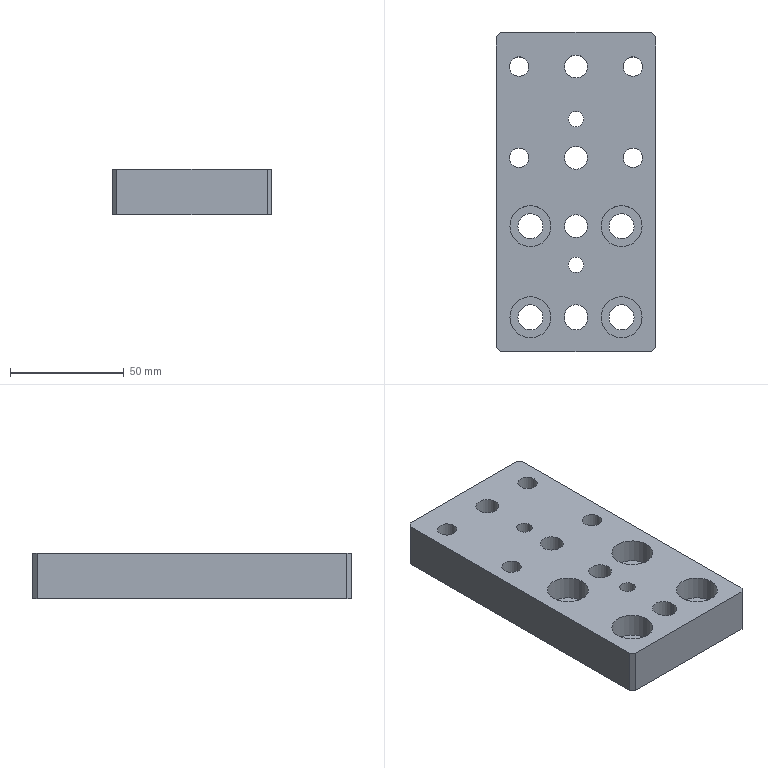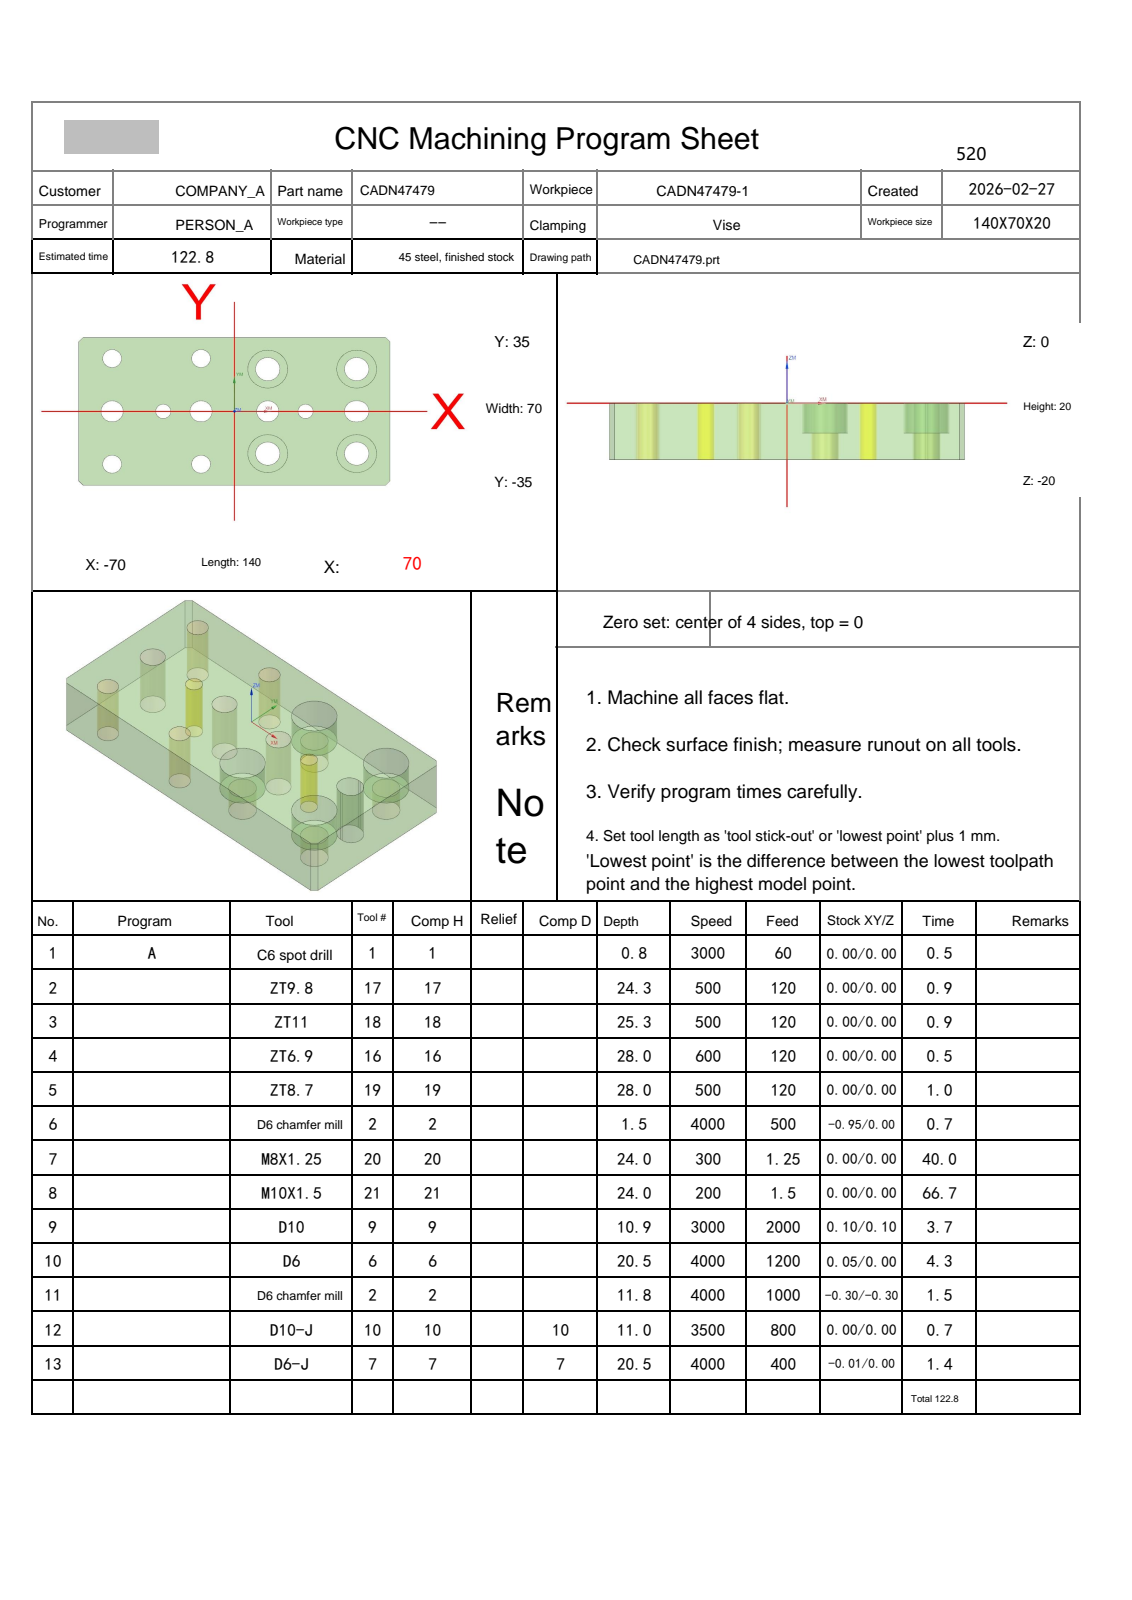NC program | NX | posted by the shop | part box 70 x 140 x 20 mm
Lines 1648 to 3434 of 3634, first 1152 of 1787 lines:
N10 T06 M06
(D6  D=6. R=0. H=06 ce=0.05 di=0.00)
G00 G90 G54 X55. Y1.95 M03 S3500
G43 H06 Z30.
M08
Z.5
G01 X54.5 Z.495 F1200.
G03 X52.55 Y0.0 Z.463 I0.0 J-1.95
X54.5 Y-1.95 Z.43 I1.95 J0.0
G01 X55.5 Z.42
G03 X57.45 Y0.0 Z.388 I0.0 J1.95
X55.5 Y1.95 Z.356 I-1.95 J0.0
G01 X54.5 Z.345
G03 X52.55 Y0.0 Z.313 I0.0 J-1.95
X54.5 Y-1.95 Z.281 I1.95 J0.0
G01 X55.5 Z.27
G03 X57.45 Y0.0 Z.238 I0.0 J1.95
X55.5 Y1.95 Z.206 I-1.95 J0.0
G01 X54.5 Z.195
G03 X52.55 Y0.0 Z.163 I0.0 J-1.95
X54.5 Y-1.95 Z.131 I1.95 J0.0
G01 X55.5 Z.121
G03 X57.45 Y0.0 Z.089 I0.0 J1.95
X55.5 Y1.95 Z.056 I-1.95 J0.0
G01 X54.5 Z.046
G03 X52.55 Y0.0 Z.014 I0.0 J-1.95
X54.5 Y-1.95 Z-.018 I1.95 J0.0
G01 X55.5 Z-.029
G03 X57.45 Y0.0 Z-.061 I0.0 J1.95
X55.5 Y1.95 Z-.093 I-1.95 J0.0
G01 X54.5 Z-.104
G03 X52.55 Y0.0 Z-.136 I0.0 J-1.95
X54.5 Y-1.95 Z-.168 I1.95 J0.0
G01 X55.5 Z-.179
G03 X57.45 Y0.0 Z-.211 I0.0 J1.95
X55.5 Y1.95 Z-.243 I-1.95 J0.0
G01 X54.5 Z-.253
G03 X52.55 Y0.0 Z-.286 I0.0 J-1.95
X54.5 Y-1.95 Z-.318 I1.95 J0.0
G01 X55.5 Z-.328
G03 X57.45 Y0.0 Z-.36 I0.0 J1.95
X55.5 Y1.95 Z-.393 I-1.95 J0.0
G01 X54.5 Z-.403
G03 X52.55 Y0.0 Z-.435 I0.0 J-1.95
X54.5 Y-1.95 Z-.467 I1.95 J0.0
G01 X55.5 Z-.478
G03 X57.45 Y0.0 Z-.51 I0.0 J1.95
X55.5 Y1.95 Z-.542 I-1.95 J0.0
G01 X54.5 Z-.553
G03 X52.55 Y0.0 Z-.585 I0.0 J-1.95
X54.5 Y-1.95 Z-.617 I1.95 J0.0
G01 X55.5 Z-.628
G03 X57.45 Y0.0 Z-.66 I0.0 J1.95
X55.5 Y1.95 Z-.692 I-1.95 J0.0
G01 X54.5 Z-.702
G03 X52.55 Y0.0 Z-.734 I0.0 J-1.95
X54.5 Y-1.95 Z-.767 I1.95 J0.0
G01 X55.5 Z-.777
G03 X57.45 Y0.0 Z-.809 I0.0 J1.95
X55.5 Y1.95 Z-.841 I-1.95 J0.0
G01 X54.5 Z-.852
G03 X52.55 Y0.0 Z-.884 I0.0 J-1.95
X54.5 Y-1.95 Z-.916 I1.95 J0.0
G01 X55.5 Z-.927
G03 X57.45 Y0.0 Z-.959 I0.0 J1.95
X55.5 Y1.95 Z-.991 I-1.95 J0.0
G01 X54.5 Z-1.002
G03 X52.55 Y0.0 Z-1.034 I0.0 J-1.95
X54.5 Y-1.95 Z-1.066 I1.95 J0.0
G01 X55.5 Z-1.076
G03 X57.45 Y0.0 Z-1.109 I0.0 J1.95
X55.5 Y1.95 Z-1.141 I-1.95 J0.0
G01 X54.5 Z-1.151
G03 X52.55 Y0.0 Z-1.183 I0.0 J-1.95
X54.5 Y-1.95 Z-1.216 I1.95 J0.0
G01 X55.5 Z-1.226
G03 X57.45 Y0.0 Z-1.258 I0.0 J1.95
X55.5 Y1.95 Z-1.29 I-1.95 J0.0
G01 X54.5 Z-1.301
G03 X52.55 Y0.0 Z-1.333 I0.0 J-1.95
X54.5 Y-1.95 Z-1.365 I1.95 J0.0
G01 X55.5 Z-1.376
G03 X57.45 Y0.0 Z-1.408 I0.0 J1.95
X55.5 Y1.95 Z-1.44 I-1.95 J0.0
G01 X54.5 Z-1.451
G03 X52.55 Y0.0 Z-1.483 I0.0 J-1.95
X54.5 Y-1.95 Z-1.515 I1.95 J0.0
G01 X55.5 Z-1.525
G03 X57.45 Y0.0 Z-1.557 I0.0 J1.95
X55.5 Y1.95 Z-1.59 I-1.95 J0.0
G01 X54.5 Z-1.6
G03 X52.55 Y0.0 Z-1.632 I0.0 J-1.95
X54.5 Y-1.95 Z-1.664 I1.95 J0.0
G01 X55.5 Z-1.675
G03 X57.45 Y0.0 Z-1.707 I0.0 J1.95
X55.5 Y1.95 Z-1.739 I-1.95 J0.0
G01 X54.5 Z-1.75
G03 X52.55 Y0.0 Z-1.782 I0.0 J-1.95
X54.5 Y-1.95 Z-1.814 I1.95 J0.0
G01 X55.5 Z-1.825
G03 X57.45 Y0.0 Z-1.857 I0.0 J1.95
X55.5 Y1.95 Z-1.889 I-1.95 J0.0
G01 X54.5 Z-1.899
G03 X52.55 Y0.0 Z-1.932 I0.0 J-1.95
X54.5 Y-1.95 Z-1.964 I1.95 J0.0
G01 X55.5 Z-1.974
G03 X57.45 Y0.0 Z-2.006 I0.0 J1.95
X55.5 Y1.95 Z-2.039 I-1.95 J0.0
G01 X54.5 Z-2.049
G03 X52.55 Y0.0 Z-2.081 I0.0 J-1.95
X54.5 Y-1.95 Z-2.113 I1.95 J0.0
G01 X55.5 Z-2.124
G03 X57.45 Y0.0 Z-2.156 I0.0 J1.95
X55.5 Y1.95 Z-2.188 I-1.95 J0.0
G01 X54.5 Z-2.199
G03 X52.55 Y0.0 Z-2.231 I0.0 J-1.95
X54.5 Y-1.95 Z-2.263 I1.95 J0.0
G01 X55.5 Z-2.273
G03 X57.45 Y0.0 Z-2.306 I0.0 J1.95
X55.5 Y1.95 Z-2.338 I-1.95 J0.0
G01 X54.5 Z-2.348
G03 X52.55 Y0.0 Z-2.38 I0.0 J-1.95
X54.5 Y-1.95 Z-2.413 I1.95 J0.0
G01 X55.5 Z-2.423
G03 X57.45 Y0.0 Z-2.455 I0.0 J1.95
X55.5 Y1.95 Z-2.487 I-1.95 J0.0
G01 X54.5 Z-2.498
G03 X52.55 Y0.0 Z-2.53 I0.0 J-1.95
X54.5 Y-1.95 Z-2.562 I1.95 J0.0
G01 X55.5 Z-2.573
G03 X57.45 Y0.0 Z-2.605 I0.0 J1.95
X55.5 Y1.95 Z-2.637 I-1.95 J0.0
G01 X54.5 Z-2.648
G03 X52.55 Y0.0 Z-2.68 I0.0 J-1.95
X54.5 Y-1.95 Z-2.712 I1.95 J0.0
G01 X55.5 Z-2.722
G03 X57.45 Y0.0 Z-2.755 I0.0 J1.95
X55.5 Y1.95 Z-2.787 I-1.95 J0.0
G01 X54.5 Z-2.797
G03 X52.55 Y0.0 Z-2.829 I0.0 J-1.95
X54.5 Y-1.95 Z-2.862 I1.95 J0.0
G01 X55.5 Z-2.872
G03 X57.45 Y0.0 Z-2.904 I0.0 J1.95
X55.5 Y1.95 Z-2.936 I-1.95 J0.0
G01 X54.5 Z-2.947
G03 X52.55 Y0.0 Z-2.979 I0.0 J-1.95
X54.5 Y-1.95 Z-3.011 I1.95 J0.0
G01 X55.5 Z-3.022
G03 X57.45 Y0.0 Z-3.054 I0.0 J1.95
X55.5 Y1.95 Z-3.086 I-1.95 J0.0
G01 X54.5 Z-3.096
G03 X52.55 Y0.0 Z-3.129 I0.0 J-1.95
X54.5 Y-1.95 Z-3.161 I1.95 J0.0
G01 X55.5 Z-3.171
G03 X57.45 Y0.0 Z-3.203 I0.0 J1.95
X55.5 Y1.95 Z-3.236 I-1.95 J0.0
G01 X54.5 Z-3.246
G03 X52.55 Y0.0 Z-3.278 I0.0 J-1.95
X54.5 Y-1.95 Z-3.31 I1.95 J0.0
G01 X55.5 Z-3.321
G03 X57.45 Y0.0 Z-3.353 I0.0 J1.95
X55.5 Y1.95 Z-3.385 I-1.95 J0.0
G01 X54.5 Z-3.396
G03 X52.55 Y0.0 Z-3.428 I0.0 J-1.95
X54.5 Y-1.95 Z-3.46 I1.95 J0.0
G01 X55.5 Z-3.471
G03 X57.45 Y0.0 Z-3.503 I0.0 J1.95
X55.5 Y1.95 Z-3.535 I-1.95 J0.0
G01 X54.5 Z-3.545
G03 X52.55 Y0.0 Z-3.578 I0.0 J-1.95
X54.5 Y-1.95 Z-3.61 I1.95 J0.0
G01 X55.5 Z-3.62
G03 X57.45 Y0.0 Z-3.652 I0.0 J1.95
X55.5 Y1.95 Z-3.685 I-1.95 J0.0
G01 X54.5 Z-3.695
G03 X52.55 Y0.0 Z-3.727 I0.0 J-1.95
X54.5 Y-1.95 Z-3.759 I1.95 J0.0
G01 X55.5 Z-3.77
G03 X57.45 Y0.0 Z-3.802 I0.0 J1.95
X55.5 Y1.95 Z-3.834 I-1.95 J0.0
G01 X54.5 Z-3.845
G03 X52.55 Y0.0 Z-3.877 I0.0 J-1.95
X54.5 Y-1.95 Z-3.909 I1.95 J0.0
G01 X55.5 Z-3.919
G03 X57.45 Y0.0 Z-3.952 I0.0 J1.95
X55.5 Y1.95 Z-3.984 I-1.95 J0.0
G01 X54.5 Z-3.994
G03 X52.55 Y0.0 Z-4.026 I0.0 J-1.95
X54.5 Y-1.95 Z-4.059 I1.95 J0.0
G01 X55.5 Z-4.069
G03 X57.45 Y0.0 Z-4.101 I0.0 J1.95
X55.5 Y1.95 Z-4.133 I-1.95 J0.0
G01 X54.5 Z-4.144
G03 X52.55 Y0.0 Z-4.176 I0.0 J-1.95
X54.5 Y-1.95 Z-4.208 I1.95 J0.0
G01 X55.5 Z-4.219
G03 X57.45 Y0.0 Z-4.251 I0.0 J1.95
X55.5 Y1.95 Z-4.283 I-1.95 J0.0
G01 X54.5 Z-4.294
G03 X52.55 Y0.0 Z-4.326 I0.0 J-1.95
X54.5 Y-1.95 Z-4.358 I1.95 J0.0
G01 X55.5 Z-4.368
G03 X57.45 Y0.0 Z-4.401 I0.0 J1.95
X55.5 Y1.95 Z-4.433 I-1.95 J0.0
G01 X54.5 Z-4.443
G03 X52.55 Y0.0 Z-4.475 I0.0 J-1.95
X54.5 Y-1.95 Z-4.508 I1.95 J0.0
G01 X55.5 Z-4.518
G03 X57.45 Y0.0 Z-4.55 I0.0 J1.95
X55.5 Y1.95 Z-4.582 I-1.95 J0.0
G01 X54.5 Z-4.593
G03 X52.55 Y0.0 Z-4.625 I0.0 J-1.95
X54.5 Y-1.95 Z-4.657 I1.95 J0.0
G01 X55.5 Z-4.668
G03 X57.45 Y0.0 Z-4.7 I0.0 J1.95
X55.5 Y1.95 Z-4.732 I-1.95 J0.0
G01 X54.5 Z-4.742
G03 X52.55 Y0.0 Z-4.775 I0.0 J-1.95
X54.5 Y-1.95 Z-4.807 I1.95 J0.0
G01 X55.5 Z-4.817
G03 X57.45 Y0.0 Z-4.849 I0.0 J1.95
X55.5 Y1.95 Z-4.882 I-1.95 J0.0
G01 X54.5 Z-4.892
G03 X52.55 Y0.0 Z-4.924 I0.0 J-1.95
X54.5 Y-1.95 Z-4.956 I1.95 J0.0
G01 X55.5 Z-4.967
G03 X57.45 Y0.0 Z-4.999 I0.0 J1.95
X55.5 Y1.95 Z-5.031 I-1.95 J0.0
G01 X54.5 Z-5.042
G03 X52.55 Y0.0 Z-5.074 I0.0 J-1.95
X54.5 Y-1.95 Z-5.106 I1.95 J0.0
G01 X55.5 Z-5.117
G03 X57.45 Y0.0 Z-5.149 I0.0 J1.95
X55.5 Y1.95 Z-5.181 I-1.95 J0.0
G01 X54.5 Z-5.191
G03 X52.55 Y0.0 Z-5.224 I0.0 J-1.95
X54.5 Y-1.95 Z-5.256 I1.95 J0.0
G01 X55.5 Z-5.266
G03 X57.45 Y0.0 Z-5.298 I0.0 J1.95
X55.5 Y1.95 Z-5.331 I-1.95 J0.0
G01 X54.5 Z-5.341
G03 X52.55 Y0.0 Z-5.373 I0.0 J-1.95
X54.5 Y-1.95 Z-5.405 I1.95 J0.0
G01 X55.5 Z-5.416
G03 X57.45 Y0.0 Z-5.448 I0.0 J1.95
X55.5 Y1.95 Z-5.48 I-1.95 J0.0
G01 X54.5 Z-5.491
G03 X52.55 Y0.0 Z-5.523 I0.0 J-1.95
X54.5 Y-1.95 Z-5.555 I1.95 J0.0
G01 X55.5 Z-5.565
G03 X57.45 Y0.0 Z-5.598 I0.0 J1.95
X55.5 Y1.95 Z-5.63 I-1.95 J0.0
G01 X54.5 Z-5.64
G03 X52.55 Y0.0 Z-5.672 I0.0 J-1.95
X54.5 Y-1.95 Z-5.705 I1.95 J0.0
G01 X55.5 Z-5.715
G03 X57.45 Y0.0 Z-5.747 I0.0 J1.95
X55.5 Y1.95 Z-5.779 I-1.95 J0.0
G01 X54.5 Z-5.79
G03 X52.55 Y0.0 Z-5.822 I0.0 J-1.95
X54.5 Y-1.95 Z-5.854 I1.95 J0.0
G01 X55.5 Z-5.865
G03 X57.45 Y0.0 Z-5.897 I0.0 J1.95
X55.5 Y1.95 Z-5.929 I-1.95 J0.0
G01 X54.5 Z-5.94
G03 X52.55 Y0.0 Z-5.972 I0.0 J-1.95
X54.5 Y-1.95 Z-6.004 I1.95 J0.0
G01 X55.5 Z-6.014
G03 X57.45 Y0.0 Z-6.047 I0.0 J1.95
X55.5 Y1.95 Z-6.079 I-1.95 J0.0
G01 X54.5 Z-6.089
G03 X52.55 Y0.0 Z-6.121 I0.0 J-1.95
X54.5 Y-1.95 Z-6.154 I1.95 J0.0
G01 X55.5 Z-6.164
G03 X57.45 Y0.0 Z-6.196 I0.0 J1.95
X55.5 Y1.95 Z-6.228 I-1.95 J0.0
G01 X54.5 Z-6.239
G03 X52.55 Y0.0 Z-6.271 I0.0 J-1.95
X54.5 Y-1.95 Z-6.303 I1.95 J0.0
G01 X55.5 Z-6.314
G03 X57.45 Y0.0 Z-6.346 I0.0 J1.95
X55.5 Y1.95 Z-6.378 I-1.95 J0.0
G01 X54.5 Z-6.388
G03 X52.55 Y0.0 Z-6.421 I0.0 J-1.95
X54.5 Y-1.95 Z-6.453 I1.95 J0.0
G01 X55.5 Z-6.463
G03 X57.45 Y0.0 Z-6.495 I0.0 J1.95
X55.5 Y1.95 Z-6.528 I-1.95 J0.0
G01 X54.5 Z-6.538
G03 X52.55 Y0.0 Z-6.57 I0.0 J-1.95
X54.5 Y-1.95 Z-6.602 I1.95 J0.0
G01 X55.5 Z-6.613
G03 X57.45 Y0.0 Z-6.645 I0.0 J1.95
X55.5 Y1.95 Z-6.677 I-1.95 J0.0
G01 X54.5 Z-6.688
G03 X52.55 Y0.0 Z-6.72 I0.0 J-1.95
X54.5 Y-1.95 Z-6.752 I1.95 J0.0
G01 X55.5 Z-6.763
G03 X57.45 Y0.0 Z-6.795 I0.0 J1.95
X55.5 Y1.95 Z-6.827 I-1.95 J0.0
G01 X54.5 Z-6.837
G03 X52.55 Y0.0 Z-6.87 I0.0 J-1.95
X54.5 Y-1.95 Z-6.902 I1.95 J0.0
G01 X55.5 Z-6.912
G03 X57.45 Y0.0 Z-6.944 I0.0 J1.95
X55.5 Y1.95 Z-6.977 I-1.95 J0.0
G01 X54.5 Z-6.987
G03 X52.55 Y0.0 Z-7.019 I0.0 J-1.95
X54.5 Y-1.95 Z-7.051 I1.95 J0.0
G01 X55.5 Z-7.062
G03 X57.45 Y0.0 Z-7.094 I0.0 J1.95
X55.5 Y1.95 Z-7.126 I-1.95 J0.0
G01 X54.5 Z-7.137
G03 X52.55 Y0.0 Z-7.169 I0.0 J-1.95
X54.5 Y-1.95 Z-7.201 I1.95 J0.0
G01 X55.5 Z-7.211
G03 X57.45 Y0.0 Z-7.244 I0.0 J1.95
X55.5 Y1.95 Z-7.276 I-1.95 J0.0
G01 X54.5 Z-7.286
G03 X52.55 Y0.0 Z-7.318 I0.0 J-1.95
X54.5 Y-1.95 Z-7.351 I1.95 J0.0
G01 X55.5 Z-7.361
G03 X57.45 Y0.0 Z-7.393 I0.0 J1.95
X55.5 Y1.95 Z-7.425 I-1.95 J0.0
G01 X54.5 Z-7.436
G03 X52.55 Y0.0 Z-7.468 I0.0 J-1.95
X54.5 Y-1.95 Z-7.5 I1.95 J0.0
G01 X55.5 Z-7.511
G03 X57.45 Y0.0 Z-7.543 I0.0 J1.95
X55.5 Y1.95 Z-7.575 I-1.95 J0.0
G01 X54.5 Z-7.586
G03 X52.55 Y0.0 Z-7.618 I0.0 J-1.95
X54.5 Y-1.95 Z-7.65 I1.95 J0.0
G01 X55.5 Z-7.66
G03 X57.45 Y0.0 Z-7.693 I0.0 J1.95
X55.5 Y1.95 Z-7.725 I-1.95 J0.0
G01 X54.5 Z-7.735
G03 X52.55 Y0.0 Z-7.767 I0.0 J-1.95
X54.5 Y-1.95 Z-7.799 I1.95 J0.0
G01 X55.5 Z-7.81
G03 X57.45 Y0.0 Z-7.842 I0.0 J1.95
X55.5 Y1.95 Z-7.874 I-1.95 J0.0
G01 X54.5 Z-7.885
G03 X52.55 Y0.0 Z-7.917 I0.0 J-1.95
X54.5 Y-1.95 Z-7.949 I1.95 J0.0
G01 X55.5 Z-7.96
G03 X57.45 Y0.0 Z-7.992 I0.0 J1.95
X55.5 Y1.95 Z-8.024 I-1.95 J0.0
G01 X54.5 Z-8.034
G03 X52.55 Y0.0 Z-8.067 I0.0 J-1.95
X54.5 Y-1.95 Z-8.099 I1.95 J0.0
G01 X55.5 Z-8.109
G03 X57.45 Y0.0 Z-8.141 I0.0 J1.95
X55.5 Y1.95 Z-8.174 I-1.95 J0.0
G01 X54.5 Z-8.184
G03 X52.55 Y0.0 Z-8.216 I0.0 J-1.95
X54.5 Y-1.95 Z-8.248 I1.95 J0.0
G01 X55.5 Z-8.259
G03 X57.45 Y0.0 Z-8.291 I0.0 J1.95
X55.5 Y1.95 Z-8.323 I-1.95 J0.0
G01 X54.5 Z-8.334
G03 X52.55 Y0.0 Z-8.366 I0.0 J-1.95
X54.5 Y-1.95 Z-8.398 I1.95 J0.0
G01 X55.5 Z-8.409
G03 X57.45 Y0.0 Z-8.441 I0.0 J1.95
X55.5 Y1.95 Z-8.473 I-1.95 J0.0
G01 X54.5 Z-8.483
G03 X52.55 Y0.0 Z-8.516 I0.0 J-1.95
X54.5 Y-1.95 Z-8.548 I1.95 J0.0
G01 X55.5 Z-8.558
G03 X57.45 Y0.0 Z-8.59 I0.0 J1.95
X55.5 Y1.95 Z-8.622 I-1.95 J0.0
G01 X54.5 Z-8.633
G03 X52.55 Y0.0 Z-8.665 I0.0 J-1.95
X54.5 Y-1.95 Z-8.697 I1.95 J0.0
G01 X55.5 Z-8.708
G03 X57.45 Y0.0 Z-8.74 I0.0 J1.95
X55.5 Y1.95 Z-8.772 I-1.95 J0.0
G01 X54.5 Z-8.783
G03 X52.55 Y0.0 Z-8.815 I0.0 J-1.95
X54.5 Y-1.95 Z-8.847 I1.95 J0.0
G01 X55.5 Z-8.857
G03 X57.45 Y0.0 Z-8.89 I0.0 J1.95
X55.5 Y1.95 Z-8.922 I-1.95 J0.0
G01 X54.5 Z-8.932
G03 X52.55 Y0.0 Z-8.964 I0.0 J-1.95
X54.5 Y-1.95 Z-8.997 I1.95 J0.0
G01 X55.5 Z-9.007
G03 X57.45 Y0.0 Z-9.039 I0.0 J1.95
X55.5 Y1.95 Z-9.071 I-1.95 J0.0
G01 X54.5 Z-9.082
G03 X52.55 Y0.0 Z-9.114 I0.0 J-1.95
X54.5 Y-1.95 Z-9.146 I1.95 J0.0
G01 X55.5 Z-9.157
G03 X57.45 Y0.0 Z-9.189 I0.0 J1.95
X55.5 Y1.95 Z-9.221 I-1.95 J0.0
G01 X54.5 Z-9.232
G03 X52.55 Y0.0 Z-9.264 I0.0 J-1.95
X54.5 Y-1.95 Z-9.296 I1.95 J0.0
G01 X55.5 Z-9.306
G03 X57.45 Y0.0 Z-9.339 I0.0 J1.95
X55.5 Y1.95 Z-9.371 I-1.95 J0.0
G01 X54.5 Z-9.381
G03 X52.55 Y0.0 Z-9.413 I0.0 J-1.95
X54.5 Y-1.95 Z-9.445 I1.95 J0.0
G01 X55.5 Z-9.456
G03 X57.45 Y0.0 Z-9.488 I0.0 J1.95
X55.5 Y1.95 Z-9.52 I-1.95 J0.0
G01 X54.5 Z-9.531
G03 X52.55 Y0.0 Z-9.563 I0.0 J-1.95
X54.5 Y-1.95 Z-9.595 I1.95 J0.0
G01 X55.5 Z-9.606
G03 X57.45 Y0.0 Z-9.638 I0.0 J1.95
X55.5 Y1.95 Z-9.67 I-1.95 J0.0
G01 X54.5 Z-9.68
G03 X52.55 Y0.0 Z-9.713 I0.0 J-1.95
X54.5 Y-1.95 Z-9.745 I1.95 J0.0
G01 X55.5 Z-9.755
G03 X57.45 Y0.0 Z-9.787 I0.0 J1.95
X55.5 Y1.95 Z-9.82 I-1.95 J0.0
G01 X54.5 Z-9.83
G03 X52.55 Y0.0 Z-9.862 I0.0 J-1.95
X54.5 Y-1.95 Z-9.894 I1.95 J0.0
G01 X55.5 Z-9.905
G03 X57.45 Y0.0 Z-9.937 I0.0 J1.95
X55.5 Y1.95 Z-9.969 I-1.95 J0.0
G01 X54.5 Z-9.98
G03 X52.55 Y0.0 Z-10.012 I0.0 J-1.95
X54.5 Y-1.95 Z-10.044 I1.95 J0.0
G01 X55.5 Z-10.055
G03 X57.45 Y0.0 Z-10.087 I0.0 J1.95
X55.5 Y1.95 Z-10.119 I-1.95 J0.0
G01 X54.5 Z-10.129
G03 X52.55 Y0.0 Z-10.161 I0.0 J-1.95
X54.5 Y-1.95 Z-10.194 I1.95 J0.0
G01 X55.5 Z-10.204
G03 X57.45 Y0.0 Z-10.236 I0.0 J1.95
X55.5 Y1.95 Z-10.268 I-1.95 J0.0
G01 X54.5 Z-10.279
G03 X52.55 Y0.0 Z-10.311 I0.0 J-1.95
X54.5 Y-1.95 Z-10.343 I1.95 J0.0
G01 X55.5 Z-10.354
G03 X57.45 Y0.0 Z-10.386 I0.0 J1.95
X55.5 Y1.95 Z-10.418 I-1.95 J0.0
G01 X54.5 Z-10.429
G03 X52.55 Y0.0 Z-10.461 I0.0 J-1.95
X54.5 Y-1.95 Z-10.493 I1.95 J0.0
G01 X55.5 Z-10.503
G03 X57.45 Y0.0 Z-10.536 I0.0 J1.95
X55.5 Y1.95 Z-10.568 I-1.95 J0.0
G01 X54.5 Z-10.578
G03 X52.55 Y0.0 Z-10.61 I0.0 J-1.95
X54.5 Y-1.95 Z-10.643 I1.95 J0.0
G01 X55.5 Z-10.653
G03 X57.45 Y0.0 Z-10.685 I0.0 J1.95
X55.5 Y1.95 Z-10.717 I-1.95 J0.0
G01 X54.5 Z-10.728
G03 X52.55 Y0.0 Z-10.76 I0.0 J-1.95
X54.5 Y-1.95 Z-10.792 I1.95 J0.0
G01 X55.5 Z-10.803
G03 X57.45 Y0.0 Z-10.835 I0.0 J1.95
X55.5 Y1.95 Z-10.867 I-1.95 J0.0
G01 X54.5 Z-10.878
G03 X52.55 Y0.0 Z-10.91 I0.0 J-1.95
X54.5 Y-1.95 Z-10.942 I1.95 J0.0
G01 X55.5 Z-10.952
G03 X57.45 Y0.0 Z-10.984 I0.0 J1.95
X55.5 Y1.95 Z-11.017 I-1.95 J0.0
G01 X54.5 Z-11.027
G03 X52.55 Y0.0 Z-11.059 I0.0 J-1.95
X54.5 Y-1.95 Z-11.091 I1.95 J0.0
G01 X55.5 Z-11.102
G03 X57.45 Y0.0 Z-11.134 I0.0 J1.95
X55.5 Y1.95 Z-11.166 I-1.95 J0.0
G01 X54.5 Z-11.177
G03 X52.55 Y0.0 Z-11.209 I0.0 J-1.95
X54.5 Y-1.95 Z-11.241 I1.95 J0.0
G01 X55.5 Z-11.252
G03 X57.45 Y0.0 Z-11.284 I0.0 J1.95
X55.5 Y1.95 Z-11.316 I-1.95 J0.0
G01 X54.5 Z-11.326
G03 X52.55 Y0.0 Z-11.359 I0.0 J-1.95
X54.5 Y-1.95 Z-11.391 I1.95 J0.0
G01 X55.5 Z-11.401
G03 X57.45 Y0.0 Z-11.433 I0.0 J1.95
X55.5 Y1.95 Z-11.466 I-1.95 J0.0
G01 X54.5 Z-11.476
G03 X52.55 Y0.0 Z-11.508 I0.0 J-1.95
X54.5 Y-1.95 Z-11.54 I1.95 J0.0
G01 X55.5 Z-11.551
G03 X57.45 Y0.0 Z-11.583 I0.0 J1.95
X55.5 Y1.95 Z-11.615 I-1.95 J0.0
G01 X54.5 Z-11.626
G03 X52.55 Y0.0 Z-11.658 I0.0 J-1.95
X54.5 Y-1.95 Z-11.69 I1.95 J0.0
G01 X55.5 Z-11.701
G03 X57.45 Y0.0 Z-11.733 I0.0 J1.95
X55.5 Y1.95 Z-11.765 I-1.95 J0.0
G01 X54.5 Z-11.775
G03 X52.55 Y0.0 Z-11.807 I0.0 J-1.95
X54.5 Y-1.95 Z-11.84 I1.95 J0.0
G01 X55.5 Z-11.85
G03 X57.45 Y0.0 Z-11.882 I0.0 J1.95
X55.5 Y1.95 Z-11.914 I-1.95 J0.0
G01 X54.5 Z-11.925
G03 X52.55 Y0.0 Z-11.957 I0.0 J-1.95
X54.5 Y-1.95 Z-11.989 I1.95 J0.0
G01 X55.5 Z-12.
G03 X57.45 Y0.0 Z-12.032 I0.0 J1.95
X55.5 Y1.95 Z-12.064 I-1.95 J0.0
G01 X54.5 Z-12.075
G03 X52.55 Y0.0 Z-12.107 I0.0 J-1.95
X54.5 Y-1.95 Z-12.139 I1.95 J0.0
G01 X55.5 Z-12.149
G03 X57.45 Y0.0 Z-12.182 I0.0 J1.95
X55.5 Y1.95 Z-12.214 I-1.95 J0.0
G01 X54.5 Z-12.224
G03 X52.55 Y0.0 Z-12.256 I0.0 J-1.95
X54.5 Y-1.95 Z-12.289 I1.95 J0.0
G01 X55.5 Z-12.299
G03 X57.45 Y0.0 Z-12.331 I0.0 J1.95
X55.5 Y1.95 Z-12.363 I-1.95 J0.0
G01 X54.5 Z-12.374
G03 X52.55 Y0.0 Z-12.406 I0.0 J-1.95
X54.5 Y-1.95 Z-12.438 I1.95 J0.0
G01 X55.5 Z-12.449
G03 X57.45 Y0.0 Z-12.481 I0.0 J1.95
X55.5 Y1.95 Z-12.513 I-1.95 J0.0
G01 X54.5 Z-12.523
G03 X52.55 Y0.0 Z-12.556 I0.0 J-1.95
X54.5 Y-1.95 Z-12.588 I1.95 J0.0
G01 X55.5 Z-12.598
G03 X57.45 Y0.0 Z-12.63 I0.0 J1.95
X55.5 Y1.95 Z-12.663 I-1.95 J0.0
G01 X54.5 Z-12.673
G03 X52.55 Y0.0 Z-12.705 I0.0 J-1.95
X54.5 Y-1.95 Z-12.737 I1.95 J0.0
G01 X55.5 Z-12.748
G03 X57.45 Y0.0 Z-12.78 I0.0 J1.95
X55.5 Y1.95 Z-12.812 I-1.95 J0.0
G01 X54.5 Z-12.823
G03 X52.55 Y0.0 Z-12.855 I0.0 J-1.95
X54.5 Y-1.95 Z-12.887 I1.95 J0.0
G01 X55.5 Z-12.898
G03 X57.45 Y0.0 Z-12.93 I0.0 J1.95
X55.5 Y1.95 Z-12.962 I-1.95 J0.0
G01 X54.5 Z-12.972
G03 X52.55 Y0.0 Z-13.005 I0.0 J-1.95
X54.5 Y-1.95 Z-13.037 I1.95 J0.0
G01 X55.5 Z-13.047
G03 X57.45 Y0.0 Z-13.079 I0.0 J1.95
X55.5 Y1.95 Z-13.112 I-1.95 J0.0
G01 X54.5 Z-13.122
G03 X52.55 Y0.0 Z-13.154 I0.0 J-1.95
X54.5 Y-1.95 Z-13.186 I1.95 J0.0
G01 X55.5 Z-13.197
G03 X57.45 Y0.0 Z-13.229 I0.0 J1.95
X55.5 Y1.95 Z-13.261 I-1.95 J0.0
G01 X54.5 Z-13.272
G03 X52.55 Y0.0 Z-13.304 I0.0 J-1.95
X54.5 Y-1.95 Z-13.336 I1.95 J0.0
G01 X55.5 Z-13.346
G03 X57.45 Y0.0 Z-13.379 I0.0 J1.95
X55.5 Y1.95 Z-13.411 I-1.95 J0.0
G01 X54.5 Z-13.421
G03 X52.55 Y0.0 Z-13.453 I0.0 J-1.95
X54.5 Y-1.95 Z-13.486 I1.95 J0.0
G01 X55.5 Z-13.496
G03 X57.45 Y0.0 Z-13.528 I0.0 J1.95
X55.5 Y1.95 Z-13.56 I-1.95 J0.0
G01 X54.5 Z-13.571
G03 X52.55 Y0.0 Z-13.603 I0.0 J-1.95
X54.5 Y-1.95 Z-13.635 I1.95 J0.0
G01 X55.5 Z-13.646
G03 X57.45 Y0.0 Z-13.678 I0.0 J1.95
X55.5 Y1.95 Z-13.71 I-1.95 J0.0
G01 X54.5 Z-13.721
G03 X52.55 Y0.0 Z-13.753 I0.0 J-1.95
X54.5 Y-1.95 Z-13.785 I1.95 J0.0
G01 X55.5 Z-13.795
G03 X57.45 Y0.0 Z-13.828 I0.0 J1.95
X55.5 Y1.95 Z-13.86 I-1.95 J0.0
G01 X54.5 Z-13.87
G03 X52.55 Y0.0 Z-13.902 I0.0 J-1.95
X54.5 Y-1.95 Z-13.935 I1.95 J0.0
G01 X55.5 Z-13.945
G03 X57.45 Y0.0 Z-13.977 I0.0 J1.95
X55.5 Y1.95 Z-14.009 I-1.95 J0.0
G01 X54.5 Z-14.02
G03 X52.55 Y0.0 Z-14.052 I0.0 J-1.95
X54.5 Y-1.95 Z-14.084 I1.95 J0.0
G01 X55.5 Z-14.095
G03 X57.45 Y0.0 Z-14.127 I0.0 J1.95
X55.5 Y1.95 Z-14.159 I-1.95 J0.0
G01 X54.5 Z-14.169
G03 X52.55 Y0.0 Z-14.202 I0.0 J-1.95
X54.5 Y-1.95 Z-14.234 I1.95 J0.0
G01 X55.5 Z-14.244
G03 X57.45 Y0.0 Z-14.276 I0.0 J1.95
X55.5 Y1.95 Z-14.309 I-1.95 J0.0
G01 X54.5 Z-14.319
G03 X52.55 Y0.0 Z-14.351 I0.0 J-1.95
X54.5 Y-1.95 Z-14.383 I1.95 J0.0
G01 X55.5 Z-14.394
G03 X57.45 Y0.0 Z-14.426 I0.0 J1.95
X55.5 Y1.95 Z-14.458 I-1.95 J0.0
G01 X54.5 Z-14.469
G03 X52.55 Y0.0 Z-14.501 I0.0 J-1.95
X54.5 Y-1.95 Z-14.533 I1.95 J0.0
G01 X55.5 Z-14.544
G03 X57.45 Y0.0 Z-14.576 I0.0 J1.95
X55.5 Y1.95 Z-14.608 I-1.95 J0.0
G01 X54.5 Z-14.618
G03 X52.55 Y0.0 Z-14.651 I0.0 J-1.95
X54.5 Y-1.95 Z-14.683 I1.95 J0.0
G01 X55.5 Z-14.693
G03 X57.45 Y0.0 Z-14.725 I0.0 J1.95
X55.5 Y1.95 Z-14.758 I-1.95 J0.0
G01 X54.5 Z-14.768
G03 X52.55 Y0.0 Z-14.8 I0.0 J-1.95
X54.5 Y-1.95 Z-14.832 I1.95 J0.0
G01 X55.5 Z-14.843
G03 X57.45 Y0.0 Z-14.875 I0.0 J1.95
X55.5 Y1.95 Z-14.907 I-1.95 J0.0
G01 X54.5 Z-14.918
G03 X52.55 Y0.0 Z-14.95 I0.0 J-1.95
X54.5 Y-1.95 Z-14.982 I1.95 J0.0
G01 X55.5 Z-14.992
G03 X57.45 Y0.0 Z-15.025 I0.0 J1.95
X55.5 Y1.95 Z-15.057 I-1.95 J0.0
G01 X54.5 Z-15.067
G03 X52.55 Y0.0 Z-15.099 I0.0 J-1.95
X54.5 Y-1.95 Z-15.132 I1.95 J0.0
G01 X55.5 Z-15.142
G03 X57.45 Y0.0 Z-15.174 I0.0 J1.95
X55.5 Y1.95 Z-15.206 I-1.95 J0.0
G01 X54.5 Z-15.217
G03 X52.55 Y0.0 Z-15.249 I0.0 J-1.95
X54.5 Y-1.95 Z-15.281 I1.95 J0.0
G01 X55.5 Z-15.292
G03 X57.45 Y0.0 Z-15.324 I0.0 J1.95
X55.5 Y1.95 Z-15.356 I-1.95 J0.0
G01 X54.5 Z-15.367
G03 X52.55 Y0.0 Z-15.399 I0.0 J-1.95
X54.5 Y-1.95 Z-15.431 I1.95 J0.0
G01 X55.5 Z-15.441
G03 X57.45 Y0.0 Z-15.474 I0.0 J1.95
X55.5 Y1.95 Z-15.506 I-1.95 J0.0
G01 X54.5 Z-15.516
G03 X52.55 Y0.0 Z-15.548 I0.0 J-1.95
X54.5 Y-1.95 Z-15.581 I1.95 J0.0
G01 X55.5 Z-15.591
G03 X57.45 Y0.0 Z-15.623 I0.0 J1.95
X55.5 Y1.95 Z-15.655 I-1.95 J0.0
G01 X54.5 Z-15.666
G03 X52.55 Y0.0 Z-15.698 I0.0 J-1.95
X54.5 Y-1.95 Z-15.73 I1.95 J0.0
G01 X55.5 Z-15.741
G03 X57.45 Y0.0 Z-15.773 I0.0 J1.95
X55.5 Y1.95 Z-15.805 I-1.95 J0.0
G01 X54.5 Z-15.815
G03 X52.55 Y0.0 Z-15.848 I0.0 J-1.95
X54.5 Y-1.95 Z-15.88 I1.95 J0.0
G01 X55.5 Z-15.89
G03 X57.45 Y0.0 Z-15.922 I0.0 J1.95
X55.5 Y1.95 Z-15.955 I-1.95 J0.0
G01 X54.5 Z-15.965
G03 X52.55 Y0.0 Z-15.997 I0.0 J-1.95
X54.5 Y-1.95 Z-16.029 I1.95 J0.0
G01 X55.5 Z-16.04
G03 X57.45 Y0.0 Z-16.072 I0.0 J1.95
X55.5 Y1.95 Z-16.104 I-1.95 J0.0
G01 X54.5 Z-16.115
G03 X52.55 Y0.0 Z-16.147 I0.0 J-1.95
X54.5 Y-1.95 Z-16.179 I1.95 J0.0
G01 X55.5 Z-16.19
G03 X57.45 Y0.0 Z-16.222 I0.0 J1.95
X55.5 Y1.95 Z-16.254 I-1.95 J0.0
G01 X54.5 Z-16.264
G03 X52.55 Y0.0 Z-16.297 I0.0 J-1.95
X54.5 Y-1.95 Z-16.329 I1.95 J0.0
G01 X55.5 Z-16.339
G03 X57.45 Y0.0 Z-16.371 I0.0 J1.95
X55.5 Y1.95 Z-16.404 I-1.95 J0.0
G01 X54.5 Z-16.414
G03 X52.55 Y0.0 Z-16.446 I0.0 J-1.95
X54.5 Y-1.95 Z-16.478 I1.95 J0.0
G01 X55.5 Z-16.489
G03 X57.45 Y0.0 Z-16.521 I0.0 J1.95
X55.5 Y1.95 Z-16.553 I-1.95 J0.0
G01 X54.5 Z-16.564
G03 X52.55 Y0.0 Z-16.596 I0.0 J-1.95
X54.5 Y-1.95 Z-16.628 I1.95 J0.0
G01 X55.5 Z-16.638
G03 X57.45 Y0.0 Z-16.671 I0.0 J1.95
X55.5 Y1.95 Z-16.703 I-1.95 J0.0
G01 X54.5 Z-16.713
G03 X52.55 Y0.0 Z-16.745 I0.0 J-1.95
X54.5 Y-1.95 Z-16.778 I1.95 J0.0
G01 X55.5 Z-16.788
G03 X57.45 Y0.0 Z-16.82 I0.0 J1.95
X55.5 Y1.95 Z-16.852 I-1.95 J0.0
G01 X54.5 Z-16.863
G03 X52.55 Y0.0 Z-16.895 I0.0 J-1.95
X54.5 Y-1.95 Z-16.927 I1.95 J0.0
G01 X55.5 Z-16.938
G03 X57.45 Y0.0 Z-16.97 I0.0 J1.95
X55.5 Y1.95 Z-17.002 I-1.95 J0.0
G01 X54.5 Z-17.013
G03 X52.55 Y0.0 Z-17.045 I0.0 J-1.95
X54.5 Y-1.95 Z-17.077 I1.95 J0.0
G01 X55.5 Z-17.087
G03 X57.45 Y0.0 Z-17.12 I0.0 J1.95
X55.5 Y1.95 Z-17.152 I-1.95 J0.0
G01 X54.5 Z-17.162
G03 X52.55 Y0.0 Z-17.194 I0.0 J-1.95
X54.5 Y-1.95 Z-17.227 I1.95 J0.0
G01 X55.5 Z-17.237
G03 X57.45 Y0.0 Z-17.269 I0.0 J1.95
X55.5 Y1.95 Z-17.301 I-1.95 J0.0
G01 X54.5 Z-17.312
G03 X52.55 Y0.0 Z-17.344 I0.0 J-1.95
X54.5 Y-1.95 Z-17.376 I1.95 J0.0
G01 X55.5 Z-17.387
G03 X57.45 Y0.0 Z-17.419 I0.0 J1.95
X55.5 Y1.95 Z-17.451 I-1.95 J0.0
G01 X54.5 Z-17.461
G03 X52.55 Y0.0 Z-17.494 I0.0 J-1.95
X54.5 Y-1.95 Z-17.526 I1.95 J0.0
G01 X55.5 Z-17.536
G03 X57.45 Y0.0 Z-17.568 I0.0 J1.95
X55.5 Y1.95 Z-17.601 I-1.95 J0.0
G01 X54.5 Z-17.611
G03 X52.55 Y0.0 Z-17.643 I0.0 J-1.95
X54.5 Y-1.95 Z-17.675 I1.95 J0.0
G01 X55.5 Z-17.686
G03 X57.45 Y0.0 Z-17.718 I0.0 J1.95
X55.5 Y1.95 Z-17.75 I-1.95 J0.0
G01 X54.5 Z-17.761
G03 X52.55 Y0.0 Z-17.793 I0.0 J-1.95
X54.5 Y-1.95 Z-17.825 I1.95 J0.0
G01 X55.5 Z-17.836
G03 X57.45 Y0.0 Z-17.868 I0.0 J1.95
X55.5 Y1.95 Z-17.9 I-1.95 J0.0
G01 X54.5 Z-17.91
G03 X52.55 Y0.0 Z-17.943 I0.0 J-1.95
X54.5 Y-1.95 Z-17.975 I1.95 J0.0
G01 X55.5 Z-17.985
G03 X57.45 Y0.0 Z-18.017 I0.0 J1.95
X55.5 Y1.95 Z-18.049 I-1.95 J0.0
G01 X54.5 Z-18.06
G03 X52.55 Y0.0 Z-18.092 I0.0 J-1.95
X54.5 Y-1.95 Z-18.124 I1.95 J0.0
G01 X55.5 Z-18.135
G03 X57.45 Y0.0 Z-18.167 I0.0 J1.95
X55.5 Y1.95 Z-18.199 I-1.95 J0.0
G01 X54.5 Z-18.21
G03 X52.55 Y0.0 Z-18.242 I0.0 J-1.95
X54.5 Y-1.95 Z-18.274 I1.95 J0.0
G01 X55.5 Z-18.284
G03 X57.45 Y0.0 Z-18.317 I0.0 J1.95
X55.5 Y1.95 Z-18.349 I-1.95 J0.0
G01 X54.5 Z-18.359
G03 X52.55 Y0.0 Z-18.391 I0.0 J-1.95
X54.5 Y-1.95 Z-18.424 I1.95 J0.0
G01 X55.5 Z-18.434
G03 X57.45 Y0.0 Z-18.466 I0.0 J1.95
X55.5 Y1.95 Z-18.498 I-1.95 J0.0
G01 X54.5 Z-18.509
G03 X52.55 Y0.0 Z-18.541 I0.0 J-1.95
X54.5 Y-1.95 Z-18.573 I1.95 J0.0
G01 X55.5 Z-18.584
G03 X57.45 Y0.0 Z-18.616 I0.0 J1.95
X55.5 Y1.95 Z-18.648 I-1.95 J0.0
G01 X54.5 Z-18.659
G03 X52.55 Y0.0 Z-18.691 I0.0 J-1.95
X54.5 Y-1.95 Z-18.723 I1.95 J0.0
G01 X55.5 Z-18.733
G03 X57.45 Y0.0 Z-18.766 I0.0 J1.95
X55.5 Y1.95 Z-18.798 I-1.95 J0.0
G01 X54.5 Z-18.808
G03 X52.55 Y0.0 Z-18.84 I0.0 J-1.95
X54.5 Y-1.95 Z-18.872 I1.95 J0.0
G01 X55.5 Z-18.883
G03 X57.45 Y0.0 Z-18.915 I0.0 J1.95
X55.5 Y1.95 Z-18.947 I-1.95 J0.0
G01 X54.5 Z-18.958
G03 X52.55 Y0.0 Z-18.99 I0.0 J-1.95
X54.5 Y-1.95 Z-19.022 I1.95 J0.0
G01 X55.5 Z-19.033
G03 X57.45 Y0.0 Z-19.065 I0.0 J1.95
X55.5 Y1.95 Z-19.097 I-1.95 J0.0
G01 X54.5 Z-19.107
G03 X52.55 Y0.0 Z-19.14 I0.0 J-1.95
X54.5 Y-1.95 Z-19.172 I1.95 J0.0
G01 X55.5 Z-19.182
G03 X57.45 Y0.0 Z-19.214 I0.0 J1.95
X55.5 Y1.95 Z-19.247 I-1.95 J0.0
G01 X54.5 Z-19.257
G03 X52.55 Y0.0 Z-19.289 I0.0 J-1.95
X54.5 Y-1.95 Z-19.321 I1.95 J0.0
G01 X55.5 Z-19.332
G03 X57.45 Y0.0 Z-19.364 I0.0 J1.95
X55.5 Y1.95 Z-19.396 I-1.95 J0.0
G01 X54.5 Z-19.407
G03 X52.55 Y0.0 Z-19.439 I0.0 J-1.95
X54.5 Y-1.95 Z-19.471 I1.95 J0.0
G01 X55.5 Z-19.482
G03 X57.45 Y0.0 Z-19.514 I0.0 J1.95
X55.5 Y1.95 Z-19.546 I-1.95 J0.0
G01 X54.5 Z-19.556
G03 X52.55 Y0.0 Z-19.589 I0.0 J-1.95
X54.5 Y-1.95 Z-19.621 I1.95 J0.0
G01 X55.5 Z-19.631
G03 X57.45 Y0.0 Z-19.663 I0.0 J1.95
X55.5 Y1.95 Z-19.695 I-1.95 J0.0
G01 X54.5 Z-19.706
G03 X52.55 Y0.0 Z-19.738 I0.0 J-1.95
X54.5 Y-1.95 Z-19.77 I1.95 J0.0
G01 X55.5 Z-19.781
G03 X57.45 Y0.0 Z-19.813 I0.0 J1.95
X55.5 Y1.95 Z-19.845 I-1.95 J0.0
G01 X54.5 Z-19.856
G03 X52.55 Y0.0 Z-19.888 I0.0 J-1.95
X54.5 Y-1.95 Z-19.92 I1.95 J0.0
G01 X55.5 Z-19.93
G03 X57.45 Y0.0 Z-19.963 I0.0 J1.95
X55.5 Y1.95 Z-19.995 I-1.95 J0.0
G01 X55. Z-20.
X54.5
G03 X52.55 Y0.0 I0.0 J-1.95
X54.5 Y-1.95 I1.95 J0.0
G01 X55.5
G03 X57.45 Y0.0 I0.0 J1.95
X55.5 Y1.95 I-1.95 J0.0
G01 X55.
X54.5
Z-19.
G00 Z30.
G00 G90 X-55. Y0.0 M03 S4000
Z30.
Z.5
G03 X-54.03 Y.97 I0.0 J.97 F1200.
X-55. Y1.94 I-.97 J0.0
X-55. Y1.94 Z.25 I0.0 J-1.94
X-55. Y1.94 Z0.0 I0.0 J-1.94
X-55. Y1.94 Z-.25 I0.0 J-1.94
X-55. Y1.94 Z-.5 I0.0 J-1.94
X-55. Y1.94 Z-.75 I0.0 J-1.94
X-55. Y1.94 Z-1. I0.0 J-1.94
X-55. Y1.94 Z-1.25 I0.0 J-1.94
X-55. Y1.94 Z-1.5 I0.0 J-1.94
X-55. Y1.94 Z-1.75 I0.0 J-1.94
X-55. Y1.94 Z-2. I0.0 J-1.94
X-55. Y1.94 Z-2.25 I0.0 J-1.94
X-55. Y1.94 Z-2.5 I0.0 J-1.94
X-55. Y1.94 Z-2.75 I0.0 J-1.94
X-55. Y1.94 Z-3. I0.0 J-1.94
X-55. Y1.94 Z-3.25 I0.0 J-1.94
X-55. Y1.94 Z-3.5 I0.0 J-1.94
X-55. Y1.94 Z-3.75 I0.0 J-1.94
X-55. Y1.94 Z-4. I0.0 J-1.94
X-55. Y1.94 Z-4.25 I0.0 J-1.94
X-55. Y1.94 Z-4.5 I0.0 J-1.94
X-55. Y1.94 Z-4.75 I0.0 J-1.94
X-55. Y1.94 Z-5. I0.0 J-1.94
X-55. Y1.94 Z-5.25 I0.0 J-1.94
X-55. Y1.94 Z-5.5 I0.0 J-1.94
X-55. Y1.94 Z-5.75 I0.0 J-1.94
X-55. Y1.94 Z-6. I0.0 J-1.94
X-55. Y1.94 Z-6.25 I0.0 J-1.94
X-55. Y1.94 Z-6.5 I0.0 J-1.94
X-55. Y1.94 Z-6.75 I0.0 J-1.94
X-55. Y1.94 Z-7. I0.0 J-1.94
X-55. Y1.94 Z-7.25 I0.0 J-1.94
X-55. Y1.94 Z-7.5 I0.0 J-1.94
X-55. Y1.94 Z-7.75 I0.0 J-1.94
X-55. Y1.94 Z-8. I0.0 J-1.94
X-55. Y1.94 Z-8.25 I0.0 J-1.94
X-55. Y1.94 Z-8.5 I0.0 J-1.94
X-55. Y1.94 Z-8.75 I0.0 J-1.94
X-55. Y1.94 Z-9. I0.0 J-1.94
X-55. Y1.94 Z-9.25 I0.0 J-1.94
X-55. Y1.94 Z-9.5 I0.0 J-1.94
X-55. Y1.94 Z-9.75 I0.0 J-1.94
X-55. Y1.94 Z-10. I0.0 J-1.94
X-55. Y1.94 Z-10.25 I0.0 J-1.94
X-55. Y1.94 Z-10.5 I0.0 J-1.94
X-55. Y1.94 Z-10.75 I0.0 J-1.94
X-55. Y1.94 Z-11. I0.0 J-1.94
X-55. Y1.94 Z-11.25 I0.0 J-1.94
X-55. Y1.94 Z-11.5 I0.0 J-1.94
X-55. Y1.94 Z-11.75 I0.0 J-1.94
X-55. Y1.94 Z-12. I0.0 J-1.94
X-55. Y1.94 Z-12.25 I0.0 J-1.94
X-55. Y1.94 Z-12.5 I0.0 J-1.94
X-55. Y1.94 Z-12.75 I0.0 J-1.94
X-55. Y1.94 Z-13. I0.0 J-1.94
X-55. Y1.94 Z-13.25 I0.0 J-1.94
X-55. Y1.94 Z-13.5 I0.0 J-1.94
X-55. Y1.94 Z-13.75 I0.0 J-1.94
X-55. Y1.94 Z-14. I0.0 J-1.94
X-55. Y1.94 Z-14.25 I0.0 J-1.94
X-55. Y1.94 Z-14.5 I0.0 J-1.94
X-55. Y1.94 Z-14.75 I0.0 J-1.94
X-55. Y1.94 Z-15. I0.0 J-1.94
X-55. Y1.94 Z-15.25 I0.0 J-1.94
X-55. Y1.94 Z-15.5 I0.0 J-1.94
X-55. Y1.94 Z-15.75 I0.0 J-1.94
X-55. Y1.94 Z-16. I0.0 J-1.94
X-55. Y1.94 Z-16.25 I0.0 J-1.94
X-55. Y1.94 Z-16.5 I0.0 J-1.94
X-55. Y1.94 Z-16.75 I0.0 J-1.94
X-55. Y1.94 Z-17. I0.0 J-1.94
X-55. Y1.94 Z-17.25 I0.0 J-1.94
X-55. Y1.94 Z-17.5 I0.0 J-1.94
X-55. Y1.94 Z-17.75 I0.0 J-1.94
X-55. Y1.94 Z-18. I0.0 J-1.94
X-55. Y1.94 Z-18.25 I0.0 J-1.94
X-55. Y1.94 Z-18.5 I0.0 J-1.94
X-55. Y1.94 Z-18.75 I0.0 J-1.94
X-55. Y1.94 Z-19. I0.0 J-1.94
X-55. Y1.94 Z-19.25 I0.0 J-1.94
X-55. Y1.94 Z-19.5 I0.0 J-1.94
X-55. Y1.94 Z-19.75 I0.0 J-1.94
X-55. Y1.94 Z-20. I0.0 J-1.94
X-55. Y1.94 Z-20.25 I0.0 J-1.94
X-55. Y1.94 Z-20.5 I0.0 J-1.94
X-56.94 Y0.0 I0.0 J-1.94
X-55. Y-1.94 I1.94 J0.0
X-53.06 Y0.0 I0.0 J1.94
X-55. Y1.94 I-1.94 J0.0
X-55.97 Y.97 I0.0 J-.97
X-55. Y0.0 I.97 J0.0
G00 Z30.
X-15.
Z.5
G03 X-14.03 Y.97 I0.0 J.97
X-15. Y1.94 I-.97 J0.0
X-15. Y1.94 Z.25 I0.0 J-1.94
X-15. Y1.94 Z0.0 I0.0 J-1.94
X-15. Y1.94 Z-.25 I0.0 J-1.94
X-15. Y1.94 Z-.5 I0.0 J-1.94
X-15. Y1.94 Z-.75 I0.0 J-1.94
X-15. Y1.94 Z-1. I0.0 J-1.94
X-15. Y1.94 Z-1.25 I0.0 J-1.94
X-15. Y1.94 Z-1.5 I0.0 J-1.94
X-15. Y1.94 Z-1.75 I0.0 J-1.94
X-15. Y1.94 Z-2. I0.0 J-1.94
X-15. Y1.94 Z-2.25 I0.0 J-1.94
X-15. Y1.94 Z-2.5 I0.0 J-1.94
X-15. Y1.94 Z-2.75 I0.0 J-1.94
X-15. Y1.94 Z-3. I0.0 J-1.94
X-15. Y1.94 Z-3.25 I0.0 J-1.94
X-15. Y1.94 Z-3.5 I0.0 J-1.94
X-15. Y1.94 Z-3.75 I0.0 J-1.94
X-15. Y1.94 Z-4. I0.0 J-1.94
X-15. Y1.94 Z-4.25 I0.0 J-1.94
X-15. Y1.94 Z-4.5 I0.0 J-1.94
X-15. Y1.94 Z-4.75 I0.0 J-1.94
X-15. Y1.94 Z-5. I0.0 J-1.94
X-15. Y1.94 Z-5.25 I0.0 J-1.94
X-15. Y1.94 Z-5.5 I0.0 J-1.94
X-15. Y1.94 Z-5.75 I0.0 J-1.94
X-15. Y1.94 Z-6. I0.0 J-1.94
X-15. Y1.94 Z-6.25 I0.0 J-1.94
X-15. Y1.94 Z-6.5 I0.0 J-1.94
X-15. Y1.94 Z-6.75 I0.0 J-1.94
X-15. Y1.94 Z-7. I0.0 J-1.94
X-15. Y1.94 Z-7.25 I0.0 J-1.94
X-15. Y1.94 Z-7.5 I0.0 J-1.94
X-15. Y1.94 Z-7.75 I0.0 J-1.94
X-15. Y1.94 Z-8. I0.0 J-1.94
X-15. Y1.94 Z-8.25 I0.0 J-1.94
X-15. Y1.94 Z-8.5 I0.0 J-1.94
X-15. Y1.94 Z-8.75 I0.0 J-1.94
X-15. Y1.94 Z-9. I0.0 J-1.94
X-15. Y1.94 Z-9.25 I0.0 J-1.94
X-15. Y1.94 Z-9.5 I0.0 J-1.94
X-15. Y1.94 Z-9.75 I0.0 J-1.94
X-15. Y1.94 Z-10. I0.0 J-1.94
X-15. Y1.94 Z-10.25 I0.0 J-1.94
X-15. Y1.94 Z-10.5 I0.0 J-1.94
X-15. Y1.94 Z-10.75 I0.0 J-1.94
X-15. Y1.94 Z-11. I0.0 J-1.94
X-15. Y1.94 Z-11.25 I0.0 J-1.94
X-15. Y1.94 Z-11.5 I0.0 J-1.94
X-15. Y1.94 Z-11.75 I0.0 J-1.94
X-15. Y1.94 Z-12. I0.0 J-1.94
X-15. Y1.94 Z-12.25 I0.0 J-1.94
X-15. Y1.94 Z-12.5 I0.0 J-1.94
X-15. Y1.94 Z-12.75 I0.0 J-1.94
X-15. Y1.94 Z-13. I0.0 J-1.94
X-15. Y1.94 Z-13.25 I0.0 J-1.94
X-15. Y1.94 Z-13.5 I0.0 J-1.94
X-15. Y1.94 Z-13.75 I0.0 J-1.94
X-15. Y1.94 Z-14. I0.0 J-1.94
X-15. Y1.94 Z-14.25 I0.0 J-1.94
X-15. Y1.94 Z-14.5 I0.0 J-1.94
X-15. Y1.94 Z-14.75 I0.0 J-1.94
X-15. Y1.94 Z-15. I0.0 J-1.94
X-15. Y1.94 Z-15.25 I0.0 J-1.94
X-15. Y1.94 Z-15.5 I0.0 J-1.94
X-15. Y1.94 Z-15.75 I0.0 J-1.94
X-15. Y1.94 Z-16. I0.0 J-1.94
X-15. Y1.94 Z-16.25 I0.0 J-1.94
X-15. Y1.94 Z-16.5 I0.0 J-1.94
X-15. Y1.94 Z-16.75 I0.0 J-1.94
X-15. Y1.94 Z-17. I0.0 J-1.94
X-15. Y1.94 Z-17.25 I0.0 J-1.94
X-15. Y1.94 Z-17.5 I0.0 J-1.94
X-15. Y1.94 Z-17.75 I0.0 J-1.94
X-15. Y1.94 Z-18. I0.0 J-1.94
X-15. Y1.94 Z-18.25 I0.0 J-1.94
X-15. Y1.94 Z-18.5 I0.0 J-1.94
X-15. Y1.94 Z-18.75 I0.0 J-1.94
X-15. Y1.94 Z-19. I0.0 J-1.94
X-15. Y1.94 Z-19.25 I0.0 J-1.94
X-15. Y1.94 Z-19.5 I0.0 J-1.94
X-15. Y1.94 Z-19.75 I0.0 J-1.94
X-15. Y1.94 Z-20. I0.0 J-1.94
X-15. Y1.94 Z-20.25 I0.0 J-1.94
X-15. Y1.94 Z-20.5 I0.0 J-1.94
X-16.94 Y0.0 I0.0 J-1.94
X-15. Y-1.94 I1.94 J0.0
X-13.06 Y0.0 I0.0 J1.94
X-15. Y1.94 I-1.94 J0.0
X-15.97 Y.97 I0.0 J-.97
X-15. Y0.0 I.97 J0.0
G00 Z30.
X15.
Z.5
G03 X15.97 Y.97 I0.0 J.97
X15. Y1.94 I-.97 J0.0
X15. Y1.94 Z.25 I0.0 J-1.94
X15. Y1.94 Z0.0 I0.0 J-1.94
X15. Y1.94 Z-.25 I0.0 J-1.94
X15. Y1.94 Z-.5 I0.0 J-1.94
X15. Y1.94 Z-.75 I0.0 J-1.94
X15. Y1.94 Z-1. I0.0 J-1.94
X15. Y1.94 Z-1.25 I0.0 J-1.94
X15. Y1.94 Z-1.5 I0.0 J-1.94
X15. Y1.94 Z-1.75 I0.0 J-1.94
X15. Y1.94 Z-2. I0.0 J-1.94
X15. Y1.94 Z-2.25 I0.0 J-1.94
X15. Y1.94 Z-2.5 I0.0 J-1.94
X15. Y1.94 Z-2.75 I0.0 J-1.94
X15. Y1.94 Z-3. I0.0 J-1.94
X15. Y1.94 Z-3.25 I0.0 J-1.94
X15. Y1.94 Z-3.5 I0.0 J-1.94
X15. Y1.94 Z-3.75 I0.0 J-1.94
X15. Y1.94 Z-4. I0.0 J-1.94
X15. Y1.94 Z-4.25 I0.0 J-1.94
X15. Y1.94 Z-4.5 I0.0 J-1.94
X15. Y1.94 Z-4.75 I0.0 J-1.94
X15. Y1.94 Z-5. I0.0 J-1.94
X15. Y1.94 Z-5.25 I0.0 J-1.94
X15. Y1.94 Z-5.5 I0.0 J-1.94
X15. Y1.94 Z-5.75 I0.0 J-1.94
X15. Y1.94 Z-6. I0.0 J-1.94
X15. Y1.94 Z-6.25 I0.0 J-1.94
X15. Y1.94 Z-6.5 I0.0 J-1.94
X15. Y1.94 Z-6.75 I0.0 J-1.94
X15. Y1.94 Z-7. I0.0 J-1.94
X15. Y1.94 Z-7.25 I0.0 J-1.94
X15. Y1.94 Z-7.5 I0.0 J-1.94
X15. Y1.94 Z-7.75 I0.0 J-1.94
X15. Y1.94 Z-8. I0.0 J-1.94
X15. Y1.94 Z-8.25 I0.0 J-1.94
X15. Y1.94 Z-8.5 I0.0 J-1.94
X15. Y1.94 Z-8.75 I0.0 J-1.94
X15. Y1.94 Z-9. I0.0 J-1.94
X15. Y1.94 Z-9.25 I0.0 J-1.94
X15. Y1.94 Z-9.5 I0.0 J-1.94
X15. Y1.94 Z-9.75 I0.0 J-1.94
X15. Y1.94 Z-10. I0.0 J-1.94
X15. Y1.94 Z-10.25 I0.0 J-1.94
X15. Y1.94 Z-10.5 I0.0 J-1.94
X15. Y1.94 Z-10.75 I0.0 J-1.94
X15. Y1.94 Z-11. I0.0 J-1.94
X15. Y1.94 Z-11.25 I0.0 J-1.94
X15. Y1.94 Z-11.5 I0.0 J-1.94
X15. Y1.94 Z-11.75 I0.0 J-1.94
X15. Y1.94 Z-12. I0.0 J-1.94
X15. Y1.94 Z-12.25 I0.0 J-1.94
X15. Y1.94 Z-12.5 I0.0 J-1.94
X15. Y1.94 Z-12.75 I0.0 J-1.94
X15. Y1.94 Z-13. I0.0 J-1.94
X15. Y1.94 Z-13.25 I0.0 J-1.94
X15. Y1.94 Z-13.5 I0.0 J-1.94
X15. Y1.94 Z-13.75 I0.0 J-1.94
X15. Y1.94 Z-14. I0.0 J-1.94
X15. Y1.94 Z-14.25 I0.0 J-1.94
X15. Y1.94 Z-14.5 I0.0 J-1.94
X15. Y1.94 Z-14.75 I0.0 J-1.94
X15. Y1.94 Z-15. I0.0 J-1.94
X15. Y1.94 Z-15.25 I0.0 J-1.94
X15. Y1.94 Z-15.5 I0.0 J-1.94
X15. Y1.94 Z-15.75 I0.0 J-1.94
X15. Y1.94 Z-16. I0.0 J-1.94
X15. Y1.94 Z-16.25 I0.0 J-1.94
X15. Y1.94 Z-16.5 I0.0 J-1.94
X15. Y1.94 Z-16.75 I0.0 J-1.94
X15. Y1.94 Z-17. I0.0 J-1.94
X15. Y1.94 Z-17.25 I0.0 J-1.94
X15. Y1.94 Z-17.5 I0.0 J-1.94
X15. Y1.94 Z-17.75 I0.0 J-1.94
X15. Y1.94 Z-18. I0.0 J-1.94
X15. Y1.94 Z-18.25 I0.0 J-1.94
X15. Y1.94 Z-18.5 I0.0 J-1.94
X15. Y1.94 Z-18.75 I0.0 J-1.94
X15. Y1.94 Z-19. I0.0 J-1.94
X15. Y1.94 Z-19.25 I0.0 J-1.94
X15. Y1.94 Z-19.5 I0.0 J-1.94
X15. Y1.94 Z-19.75 I0.0 J-1.94
X15. Y1.94 Z-20. I0.0 J-1.94
X15. Y1.94 Z-20.25 I0.0 J-1.94
X15. Y1.94 Z-20.5 I0.0 J-1.94
X13.06 Y0.0 I0.0 J-1.94
X15. Y-1.94 I1.94 J0.0
X16.94 Y0.0 I0.0 J1.94
X15. Y1.94 I-1.94 J0.0
X14.03 Y.97 I0.0 J-.97
X15. Y0.0 I.97 J0.0
G00 Z30.
G91 G28 Z0.0
M05
M09
G91 G28 Z0.0
M01
N11 T02 M06
(D6 chamfer mill  D=6. R=0. H=02 ce=-0.30 di=0.00)
G00 G90 G54 X22.606 Y23.327 M03 S4000
G43 H02 Z30.
M08
Z2.5
G01 X22.342 Y23.877 Z2.278 F800.
X22.029 Y24.42 Z2.05
X21.675 Y24.938 Z1.821
X21.283 Y25.428 Z1.593
X20.855 Y25.887 Z1.365
X20.394 Y26.312 Z1.136
X19.902 Y26.702 Z.908
X19.382 Y27.053 Z.68
X18.837 Y27.363 Z.451
X18.27 Y27.632 Z.223
X17.684 Y27.857 Z-.005
X17.083 Y28.037 Z-.234
X16.47 Y28.172 Z-.462
X15.849 Y28.259 Z-.69
X15.223 Y28.3 Z-.919
X15. Z-1.